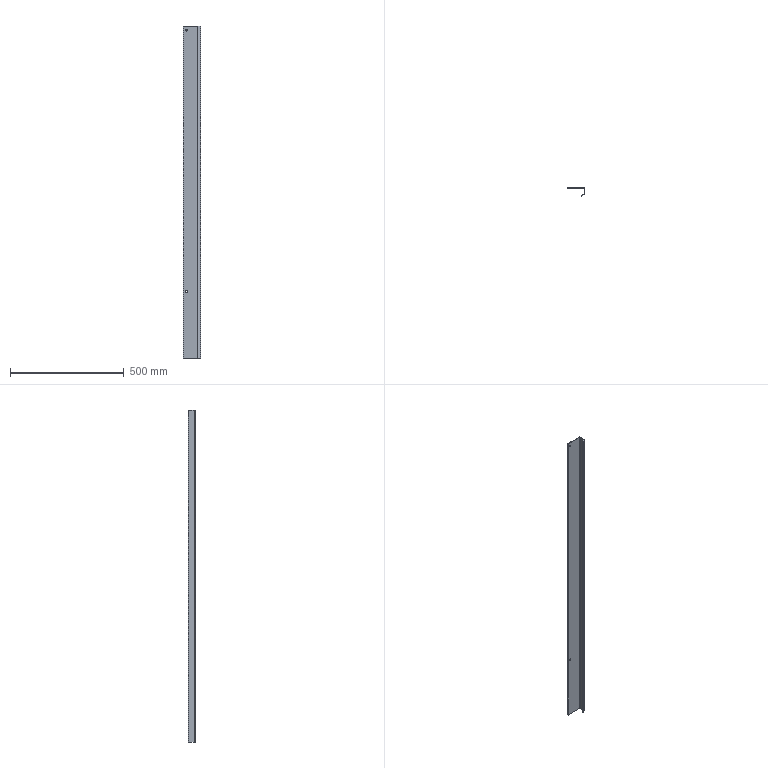Part | STEP file | Guard belt | 1 solid | 20 faces | box 75 x 33.917 x 1461 mm | volume 248061 mm3 | plane 14 | cylinder 6 | commonest cylinder face diameters 3 x2 6 x2 8.2 x2
STEP:
#1=CARTESIAN_POINT('',(0.,0.,0.));
#2=DIRECTION('',(0.,0.,1.));
#3=DIRECTION('',(1.,0.,0.));
#4=AXIS2_PLACEMENT_3D('',#1,#2,#3);
#5=CARTESIAN_POINT('',(-3.,0.,-65.));
#6=VERTEX_POINT('',#5);
#7=CARTESIAN_POINT('',(-3.,1.5,-65.));
#8=VERTEX_POINT('',#7);
#9=CARTESIAN_POINT('',(-3.,0.,-65.));
#10=DIRECTION('',(0.,1.,0.));
#11=VECTOR('',#10,1.);
#12=LINE('',#9,#11);
#13=CARTESIAN_POINT('',(0.,0.,-65.));
#14=DIRECTION('',(0.,0.,1.));
#15=DIRECTION('',(1.,0.,0.));
#16=AXIS2_PLACEMENT_3D('',#13,#14,#15);
#17=PLANE('',#16);
#18=CARTESIAN_POINT('',(-3.,0.));
#19=DIRECTION('',(0.,1.));
#20=VECTOR('',#19,1.);
#21=LINE('',#18,#20);
#22=(GEOMETRIC_REPRESENTATION_CONTEXT(2)PARAMETRIC_REPRESENTATION_CONTEXT()REPRESENTATION_CONTEXT('',''));
#23=DEFINITIONAL_REPRESENTATION('',(#21),#22);
#24=PCURVE('',#17,#23);
#25=CARTESIAN_POINT('',(0.,0.,-65.));
#26=DIRECTION('',(0.,0.,1.));
#27=DIRECTION('',(1.,0.,0.));
#28=AXIS2_PLACEMENT_3D('',#25,#26,#27);
#29=PLANE('',#28);
#30=CARTESIAN_POINT('',(-3.,0.));
#31=DIRECTION('',(0.,1.));
#32=VECTOR('',#31,1.);
#33=LINE('',#30,#32);
#34=(GEOMETRIC_REPRESENTATION_CONTEXT(2)PARAMETRIC_REPRESENTATION_CONTEXT()REPRESENTATION_CONTEXT('',''));
#35=DEFINITIONAL_REPRESENTATION('',(#33),#34);
#36=PCURVE('',#29,#35);
#37=SURFACE_CURVE('',#12,(#24,#36),.PCURVE_S1.);
#38=EDGE_CURVE('',#6,#8,#37,.T.);
#39=ORIENTED_EDGE('',*,*,#38,.F.);
#40=CARTESIAN_POINT('',(-1.5,-1.5,-65.));
#41=VERTEX_POINT('',#40);
#42=CARTESIAN_POINT('',(-3.,-1.5,-65.));
#43=DIRECTION('',(0.,0.,1.));
#44=DIRECTION('',(1.,0.,0.));
#45=AXIS2_PLACEMENT_3D('',#42,#43,#44);
#46=CIRCLE('',#45,1.5);
#47=CARTESIAN_POINT('',(-3.,-1.5));
#48=DIRECTION('',(1.,0.));
#49=AXIS2_PLACEMENT_2D('',#47,#48);
#50=CIRCLE('',#49,1.5);
#51=(GEOMETRIC_REPRESENTATION_CONTEXT(2)PARAMETRIC_REPRESENTATION_CONTEXT()REPRESENTATION_CONTEXT('',''));
#52=DEFINITIONAL_REPRESENTATION('',(#50),#51);
#53=PCURVE('',#17,#52);
#54=CARTESIAN_POINT('',(-3.,-1.5,-913.));
#55=DIRECTION('',(0.,0.,-1.));
#56=DIRECTION('',(0.,1.,0.));
#57=AXIS2_PLACEMENT_3D('',#54,#55,#56);
#58=CYLINDRICAL_SURFACE('',#57,1.5);
#59=CARTESIAN_POINT('',(1.571,-848.));
#60=DIRECTION('',(-1.,0.));
#61=VECTOR('',#60,1.);
#62=LINE('',#59,#61);
#63=(GEOMETRIC_REPRESENTATION_CONTEXT(2)PARAMETRIC_REPRESENTATION_CONTEXT()REPRESENTATION_CONTEXT('',''));
#64=DEFINITIONAL_REPRESENTATION('',(#62),#63);
#65=PCURVE('',#58,#64);
#66=SURFACE_CURVE('',#46,(#53,#65),.PCURVE_S1.);
#67=EDGE_CURVE('',#41,#6,#66,.T.);
#68=ORIENTED_EDGE('',*,*,#67,.F.);
#69=CARTESIAN_POINT('',(0.,-1.5,-65.));
#70=VERTEX_POINT('',#69);
#71=CARTESIAN_POINT('',(-1.17,-1.5,-65.));
#72=DIRECTION('',(-1.,0.,0.));
#73=VECTOR('',#72,1.);
#74=LINE('',#71,#73);
#75=CARTESIAN_POINT('',(-1.17,-1.5));
#76=DIRECTION('',(-1.,0.));
#77=VECTOR('',#76,1.);
#78=LINE('',#75,#77);
#79=(GEOMETRIC_REPRESENTATION_CONTEXT(2)PARAMETRIC_REPRESENTATION_CONTEXT()REPRESENTATION_CONTEXT('',''));
#80=DEFINITIONAL_REPRESENTATION('',(#78),#79);
#81=PCURVE('',#17,#80);
#82=CARTESIAN_POINT('',(0.,0.,-65.));
#83=DIRECTION('',(0.,0.,1.));
#84=DIRECTION('',(1.,0.,0.));
#85=AXIS2_PLACEMENT_3D('',#82,#83,#84);
#86=PLANE('',#85);
#87=CARTESIAN_POINT('',(-1.17,-1.5));
#88=DIRECTION('',(-1.,0.));
#89=VECTOR('',#88,1.);
#90=LINE('',#87,#89);
#91=(GEOMETRIC_REPRESENTATION_CONTEXT(2)PARAMETRIC_REPRESENTATION_CONTEXT()REPRESENTATION_CONTEXT('',''));
#92=DEFINITIONAL_REPRESENTATION('',(#90),#91);
#93=PCURVE('',#86,#92);
#94=SURFACE_CURVE('',#74,(#81,#93),.PCURVE_S1.);
#95=EDGE_CURVE('',#70,#41,#94,.T.);
#96=ORIENTED_EDGE('',*,*,#95,.F.);
#97=CARTESIAN_POINT('',(-3.,-1.5,-65.));
#98=DIRECTION('',(0.,0.,1.));
#99=DIRECTION('',(1.,0.,0.));
#100=AXIS2_PLACEMENT_3D('',#97,#98,#99);
#101=CIRCLE('',#100,3.);
#102=CARTESIAN_POINT('',(-3.,-1.5));
#103=DIRECTION('',(1.,0.));
#104=AXIS2_PLACEMENT_2D('',#102,#103);
#105=CIRCLE('',#104,3.);
#106=(GEOMETRIC_REPRESENTATION_CONTEXT(2)PARAMETRIC_REPRESENTATION_CONTEXT()REPRESENTATION_CONTEXT('',''));
#107=DEFINITIONAL_REPRESENTATION('',(#105),#106);
#108=PCURVE('',#17,#107);
#109=CARTESIAN_POINT('',(-3.,-1.5,-913.));
#110=DIRECTION('',(0.,0.,-1.));
#111=DIRECTION('',(0.,1.,0.));
#112=AXIS2_PLACEMENT_3D('',#109,#110,#111);
#113=CYLINDRICAL_SURFACE('',#112,3.);
#114=CARTESIAN_POINT('',(1.571,-848.));
#115=DIRECTION('',(-1.,0.));
#116=VECTOR('',#115,1.);
#117=LINE('',#114,#116);
#118=(GEOMETRIC_REPRESENTATION_CONTEXT(2)PARAMETRIC_REPRESENTATION_CONTEXT()REPRESENTATION_CONTEXT('',''));
#119=DEFINITIONAL_REPRESENTATION('',(#117),#118);
#120=PCURVE('',#113,#119);
#121=SURFACE_CURVE('',#101,(#108,#120),.PCURVE_S1.);
#122=EDGE_CURVE('',#70,#8,#121,.T.);
#123=ORIENTED_EDGE('',*,*,#122,.T.);
#124=EDGE_LOOP('',(#39,#68,#96,#123));
#125=FACE_BOUND('',#124,.T.);
#126=ADVANCED_FACE('',(#125),#17,.T.);
#127=ORIENTED_EDGE('',*,*,#38,.T.);
#128=CARTESIAN_POINT('',(-75.,1.5,-65.));
#129=VERTEX_POINT('',#128);
#130=CARTESIAN_POINT('',(0.,1.5,-65.));
#131=DIRECTION('',(-1.,0.,0.));
#132=VECTOR('',#131,1.);
#133=LINE('',#130,#132);
#134=CARTESIAN_POINT('',(0.,1.5));
#135=DIRECTION('',(-1.,0.));
#136=VECTOR('',#135,1.);
#137=LINE('',#134,#136);
#138=(GEOMETRIC_REPRESENTATION_CONTEXT(2)PARAMETRIC_REPRESENTATION_CONTEXT()REPRESENTATION_CONTEXT('',''));
#139=DEFINITIONAL_REPRESENTATION('',(#137),#138);
#140=PCURVE('',#29,#139);
#141=CARTESIAN_POINT('',(-37.5,1.5,-913.));
#142=DIRECTION('',(0.,1.,0.));
#143=DIRECTION('',(0.,0.,1.));
#144=AXIS2_PLACEMENT_3D('',#141,#142,#143);
#145=PLANE('',#144);
#146=CARTESIAN_POINT('',(848.,37.5));
#147=DIRECTION('',(0.,-1.));
#148=VECTOR('',#147,1.);
#149=LINE('',#146,#148);
#150=(GEOMETRIC_REPRESENTATION_CONTEXT(2)PARAMETRIC_REPRESENTATION_CONTEXT()REPRESENTATION_CONTEXT('',''));
#151=DEFINITIONAL_REPRESENTATION('',(#149),#150);
#152=PCURVE('',#145,#151);
#153=SURFACE_CURVE('',#133,(#140,#152),.PCURVE_S1.);
#154=EDGE_CURVE('',#8,#129,#153,.T.);
#155=ORIENTED_EDGE('',*,*,#154,.T.);
#156=CARTESIAN_POINT('',(-75.,0.,-65.));
#157=VERTEX_POINT('',#156);
#158=CARTESIAN_POINT('',(-75.,0.,-65.));
#159=DIRECTION('',(0.,1.,0.));
#160=VECTOR('',#159,1.);
#161=LINE('',#158,#160);
#162=CARTESIAN_POINT('',(-75.,0.));
#163=DIRECTION('',(0.,1.));
#164=VECTOR('',#163,1.);
#165=LINE('',#162,#164);
#166=(GEOMETRIC_REPRESENTATION_CONTEXT(2)PARAMETRIC_REPRESENTATION_CONTEXT()REPRESENTATION_CONTEXT('',''));
#167=DEFINITIONAL_REPRESENTATION('',(#165),#166);
#168=PCURVE('',#29,#167);
#169=CARTESIAN_POINT('',(-75.,0.,0.));
#170=DIRECTION('',(-1.,0.,0.));
#171=DIRECTION('',(0.,0.,1.));
#172=AXIS2_PLACEMENT_3D('',#169,#170,#171);
#173=PLANE('',#172);
#174=CARTESIAN_POINT('',(-65.,0.));
#175=DIRECTION('',(0.,1.));
#176=VECTOR('',#175,1.);
#177=LINE('',#174,#176);
#178=(GEOMETRIC_REPRESENTATION_CONTEXT(2)PARAMETRIC_REPRESENTATION_CONTEXT()REPRESENTATION_CONTEXT('',''));
#179=DEFINITIONAL_REPRESENTATION('',(#177),#178);
#180=PCURVE('',#173,#179);
#181=SURFACE_CURVE('',#161,(#168,#180),.PCURVE_S1.);
#182=EDGE_CURVE('',#157,#129,#181,.T.);
#183=ORIENTED_EDGE('',*,*,#182,.F.);
#184=CARTESIAN_POINT('',(0.,0.,-65.));
#185=DIRECTION('',(-1.,0.,0.));
#186=VECTOR('',#185,1.);
#187=LINE('',#184,#186);
#188=CARTESIAN_POINT('',(0.,0.));
#189=DIRECTION('',(-1.,0.));
#190=VECTOR('',#189,1.);
#191=LINE('',#188,#190);
#192=(GEOMETRIC_REPRESENTATION_CONTEXT(2)PARAMETRIC_REPRESENTATION_CONTEXT()REPRESENTATION_CONTEXT('',''));
#193=DEFINITIONAL_REPRESENTATION('',(#191),#192);
#194=PCURVE('',#29,#193);
#195=CARTESIAN_POINT('',(-37.5,0.,-913.));
#196=DIRECTION('',(0.,1.,0.));
#197=DIRECTION('',(0.,0.,1.));
#198=AXIS2_PLACEMENT_3D('',#195,#196,#197);
#199=PLANE('',#198);
#200=CARTESIAN_POINT('',(848.,37.5));
#201=DIRECTION('',(0.,-1.));
#202=VECTOR('',#201,1.);
#203=LINE('',#200,#202);
#204=(GEOMETRIC_REPRESENTATION_CONTEXT(2)PARAMETRIC_REPRESENTATION_CONTEXT()REPRESENTATION_CONTEXT('',''));
#205=DEFINITIONAL_REPRESENTATION('',(#203),#204);
#206=PCURVE('',#199,#205);
#207=SURFACE_CURVE('',#187,(#194,#206),.PCURVE_S1.);
#208=EDGE_CURVE('',#6,#157,#207,.T.);
#209=ORIENTED_EDGE('',*,*,#208,.F.);
#210=EDGE_LOOP('',(#127,#155,#183,#209));
#211=FACE_BOUND('',#210,.T.);
#212=ADVANCED_FACE('',(#211),#29,.T.);
#213=CARTESIAN_POINT('',(-1.5,-24.589,-65.));
#214=VERTEX_POINT('',#213);
#215=CARTESIAN_POINT('',(0.,-24.589,-65.));
#216=VERTEX_POINT('',#215);
#217=CARTESIAN_POINT('',(-1.5,-24.589,-65.));
#218=DIRECTION('',(1.,0.,0.));
#219=VECTOR('',#218,1.);
#220=LINE('',#217,#219);
#221=CARTESIAN_POINT('',(0.,0.,-65.));
#222=DIRECTION('',(0.,0.,1.));
#223=DIRECTION('',(1.,0.,0.));
#224=AXIS2_PLACEMENT_3D('',#221,#222,#223);
#225=PLANE('',#224);
#226=CARTESIAN_POINT('',(-1.5,-24.589));
#227=DIRECTION('',(1.,0.));
#228=VECTOR('',#227,1.);
#229=LINE('',#226,#228);
#230=(GEOMETRIC_REPRESENTATION_CONTEXT(2)PARAMETRIC_REPRESENTATION_CONTEXT()REPRESENTATION_CONTEXT('',''));
#231=DEFINITIONAL_REPRESENTATION('',(#229),#230);
#232=PCURVE('',#225,#231);
#233=CARTESIAN_POINT('',(-1.5,-24.589));
#234=DIRECTION('',(1.,0.));
#235=VECTOR('',#234,1.);
#236=LINE('',#233,#235);
#237=(GEOMETRIC_REPRESENTATION_CONTEXT(2)PARAMETRIC_REPRESENTATION_CONTEXT()REPRESENTATION_CONTEXT('',''));
#238=DEFINITIONAL_REPRESENTATION('',(#236),#237);
#239=PCURVE('',#86,#238);
#240=SURFACE_CURVE('',#220,(#232,#239),.PCURVE_S1.);
#241=EDGE_CURVE('',#214,#216,#240,.T.);
#242=ORIENTED_EDGE('',*,*,#241,.F.);
#243=CARTESIAN_POINT('',(-2.366,-25.948,-65.));
#244=VERTEX_POINT('',#243);
#245=CARTESIAN_POINT('',(-3.,-24.589,-65.));
#246=DIRECTION('',(0.,0.,1.));
#247=DIRECTION('',(0.4226,-0.9063,0.));
#248=AXIS2_PLACEMENT_3D('',#245,#246,#247);
#249=CIRCLE('',#248,1.5);
#250=CARTESIAN_POINT('',(-3.,-24.589));
#251=DIRECTION('',(0.4226,-0.9063));
#252=AXIS2_PLACEMENT_2D('',#250,#251);
#253=CIRCLE('',#252,1.5);
#254=(GEOMETRIC_REPRESENTATION_CONTEXT(2)PARAMETRIC_REPRESENTATION_CONTEXT()REPRESENTATION_CONTEXT('',''));
#255=DEFINITIONAL_REPRESENTATION('',(#253),#254);
#256=PCURVE('',#225,#255);
#257=CARTESIAN_POINT('',(-3.,-24.589,-913.));
#258=DIRECTION('',(0.,0.,-1.));
#259=DIRECTION('',(1.,0.,0.));
#260=AXIS2_PLACEMENT_3D('',#257,#258,#259);
#261=CYLINDRICAL_SURFACE('',#260,1.5);
#262=CARTESIAN_POINT('',(1.134,-848.));
#263=DIRECTION('',(-1.,0.));
#264=VECTOR('',#263,1.);
#265=LINE('',#262,#264);
#266=(GEOMETRIC_REPRESENTATION_CONTEXT(2)PARAMETRIC_REPRESENTATION_CONTEXT()REPRESENTATION_CONTEXT('',''));
#267=DEFINITIONAL_REPRESENTATION('',(#265),#266);
#268=PCURVE('',#261,#267);
#269=SURFACE_CURVE('',#249,(#256,#268),.PCURVE_S1.);
#270=EDGE_CURVE('',#244,#214,#269,.T.);
#271=ORIENTED_EDGE('',*,*,#270,.F.);
#272=CARTESIAN_POINT('',(-1.732,-27.308,-65.));
#273=VERTEX_POINT('',#272);
#274=CARTESIAN_POINT('',(-2.227,-26.247,-65.));
#275=DIRECTION('',(-0.4226,0.9063,0.));
#276=VECTOR('',#275,1.);
#277=LINE('',#274,#276);
#278=CARTESIAN_POINT('',(-2.227,-26.247));
#279=DIRECTION('',(-0.4226,0.9063));
#280=VECTOR('',#279,1.);
#281=LINE('',#278,#280);
#282=(GEOMETRIC_REPRESENTATION_CONTEXT(2)PARAMETRIC_REPRESENTATION_CONTEXT()REPRESENTATION_CONTEXT('',''));
#283=DEFINITIONAL_REPRESENTATION('',(#281),#282);
#284=PCURVE('',#225,#283);
#285=CARTESIAN_POINT('',(0.,0.,-65.));
#286=DIRECTION('',(0.,0.,1.));
#287=DIRECTION('',(1.,0.,0.));
#288=AXIS2_PLACEMENT_3D('',#285,#286,#287);
#289=PLANE('',#288);
#290=CARTESIAN_POINT('',(-2.227,-26.247));
#291=DIRECTION('',(-0.4226,0.9063));
#292=VECTOR('',#291,1.);
#293=LINE('',#290,#292);
#294=(GEOMETRIC_REPRESENTATION_CONTEXT(2)PARAMETRIC_REPRESENTATION_CONTEXT()REPRESENTATION_CONTEXT('',''));
#295=DEFINITIONAL_REPRESENTATION('',(#293),#294);
#296=PCURVE('',#289,#295);
#297=SURFACE_CURVE('',#277,(#284,#296),.PCURVE_S1.);
#298=EDGE_CURVE('',#273,#244,#297,.T.);
#299=ORIENTED_EDGE('',*,*,#298,.F.);
#300=CARTESIAN_POINT('',(-3.,-24.589,-65.));
#301=DIRECTION('',(0.,0.,1.));
#302=DIRECTION('',(0.4226,-0.9063,0.));
#303=AXIS2_PLACEMENT_3D('',#300,#301,#302);
#304=CIRCLE('',#303,3.);
#305=CARTESIAN_POINT('',(-3.,-24.589));
#306=DIRECTION('',(0.4226,-0.9063));
#307=AXIS2_PLACEMENT_2D('',#305,#306);
#308=CIRCLE('',#307,3.);
#309=(GEOMETRIC_REPRESENTATION_CONTEXT(2)PARAMETRIC_REPRESENTATION_CONTEXT()REPRESENTATION_CONTEXT('',''));
#310=DEFINITIONAL_REPRESENTATION('',(#308),#309);
#311=PCURVE('',#225,#310);
#312=CARTESIAN_POINT('',(-3.,-24.589,-913.));
#313=DIRECTION('',(0.,0.,-1.));
#314=DIRECTION('',(1.,0.,0.));
#315=AXIS2_PLACEMENT_3D('',#312,#313,#314);
#316=CYLINDRICAL_SURFACE('',#315,3.);
#317=CARTESIAN_POINT('',(1.134,-848.));
#318=DIRECTION('',(-1.,0.));
#319=VECTOR('',#318,1.);
#320=LINE('',#317,#319);
#321=(GEOMETRIC_REPRESENTATION_CONTEXT(2)PARAMETRIC_REPRESENTATION_CONTEXT()REPRESENTATION_CONTEXT('',''));
#322=DEFINITIONAL_REPRESENTATION('',(#320),#321);
#323=PCURVE('',#316,#322);
#324=SURFACE_CURVE('',#304,(#311,#323),.PCURVE_S1.);
#325=EDGE_CURVE('',#273,#216,#324,.T.);
#326=ORIENTED_EDGE('',*,*,#325,.T.);
#327=EDGE_LOOP('',(#242,#271,#299,#326));
#328=FACE_BOUND('',#327,.T.);
#329=ADVANCED_FACE('',(#328),#225,.T.);
#330=ORIENTED_EDGE('',*,*,#95,.T.);
#331=CARTESIAN_POINT('',(-1.5,5.286,-65.));
#332=DIRECTION('',(0.,1.,0.));
#333=VECTOR('',#332,1.);
#334=LINE('',#331,#333);
#335=CARTESIAN_POINT('',(-1.5,5.286));
#336=DIRECTION('',(0.,1.));
#337=VECTOR('',#336,1.);
#338=LINE('',#335,#337);
#339=(GEOMETRIC_REPRESENTATION_CONTEXT(2)PARAMETRIC_REPRESENTATION_CONTEXT()REPRESENTATION_CONTEXT('',''));
#340=DEFINITIONAL_REPRESENTATION('',(#338),#339);
#341=PCURVE('',#86,#340);
#342=CARTESIAN_POINT('',(-1.5,-12.304,-913.));
#343=DIRECTION('',(1.,0.,0.));
#344=DIRECTION('',(0.,0.,1.));
#345=AXIS2_PLACEMENT_3D('',#342,#343,#344);
#346=PLANE('',#345);
#347=CARTESIAN_POINT('',(848.,-17.589));
#348=DIRECTION('',(0.,-1.));
#349=VECTOR('',#348,1.);
#350=LINE('',#347,#349);
#351=(GEOMETRIC_REPRESENTATION_CONTEXT(2)PARAMETRIC_REPRESENTATION_CONTEXT()REPRESENTATION_CONTEXT('',''));
#352=DEFINITIONAL_REPRESENTATION('',(#350),#351);
#353=PCURVE('',#346,#352);
#354=SURFACE_CURVE('',#334,(#341,#353),.PCURVE_S1.);
#355=EDGE_CURVE('',#214,#41,#354,.T.);
#356=ORIENTED_EDGE('',*,*,#355,.F.);
#357=ORIENTED_EDGE('',*,*,#241,.T.);
#358=CARTESIAN_POINT('',(0.,5.286,-65.));
#359=DIRECTION('',(0.,1.,0.));
#360=VECTOR('',#359,1.);
#361=LINE('',#358,#360);
#362=CARTESIAN_POINT('',(0.,5.286));
#363=DIRECTION('',(0.,1.));
#364=VECTOR('',#363,1.);
#365=LINE('',#362,#364);
#366=(GEOMETRIC_REPRESENTATION_CONTEXT(2)PARAMETRIC_REPRESENTATION_CONTEXT()REPRESENTATION_CONTEXT('',''));
#367=DEFINITIONAL_REPRESENTATION('',(#365),#366);
#368=PCURVE('',#86,#367);
#369=CARTESIAN_POINT('',(0.,-12.304,-913.));
#370=DIRECTION('',(1.,0.,0.));
#371=DIRECTION('',(0.,0.,1.));
#372=AXIS2_PLACEMENT_3D('',#369,#370,#371);
#373=PLANE('',#372);
#374=CARTESIAN_POINT('',(848.,-17.589));
#375=DIRECTION('',(0.,-1.));
#376=VECTOR('',#375,1.);
#377=LINE('',#374,#376);
#378=(GEOMETRIC_REPRESENTATION_CONTEXT(2)PARAMETRIC_REPRESENTATION_CONTEXT()REPRESENTATION_CONTEXT('',''));
#379=DEFINITIONAL_REPRESENTATION('',(#377),#378);
#380=PCURVE('',#373,#379);
#381=SURFACE_CURVE('',#361,(#368,#380),.PCURVE_S1.);
#382=EDGE_CURVE('',#216,#70,#381,.T.);
#383=ORIENTED_EDGE('',*,*,#382,.T.);
#384=EDGE_LOOP('',(#330,#356,#357,#383));
#385=FACE_BOUND('',#384,.T.);
#386=ADVANCED_FACE('',(#385),#86,.T.);
#387=CARTESIAN_POINT('',(-57.4,0.,-1233.5));
#388=VERTEX_POINT('',#387);
#389=CARTESIAN_POINT('',(-61.5,0.,-1233.5));
#390=DIRECTION('',(0.,1.,0.));
#391=DIRECTION('',(-1.,0.,0.));
#392=AXIS2_PLACEMENT_3D('',#389,#390,#391);
#393=CIRCLE('',#392,4.1);
#394=CARTESIAN_POINT('',(-61.5,1.5,-1233.5));
#395=DIRECTION('',(0.,-1.,0.));
#396=DIRECTION('',(-1.,0.,0.));
#397=AXIS2_PLACEMENT_3D('',#394,#395,#396);
#398=CYLINDRICAL_SURFACE('',#397,4.1);
#399=CARTESIAN_POINT('',(12.566,1.5));
#400=DIRECTION('',(-1.,0.));
#401=VECTOR('',#400,1.);
#402=LINE('',#399,#401);
#403=(GEOMETRIC_REPRESENTATION_CONTEXT(2)PARAMETRIC_REPRESENTATION_CONTEXT()REPRESENTATION_CONTEXT('',''));
#404=DEFINITIONAL_REPRESENTATION('',(#402),#403);
#405=PCURVE('',#398,#404);
#406=CARTESIAN_POINT('',(-320.5,-24.));
#407=DIRECTION('',(0.,-1.));
#408=AXIS2_PLACEMENT_2D('',#406,#407);
#409=CIRCLE('',#408,4.1);
#410=(GEOMETRIC_REPRESENTATION_CONTEXT(2)PARAMETRIC_REPRESENTATION_CONTEXT()REPRESENTATION_CONTEXT('',''));
#411=DEFINITIONAL_REPRESENTATION('',(#409),#410);
#412=PCURVE('',#199,#411);
#413=SURFACE_CURVE('',#393,(#405,#412),.PCURVE_S1.);
#414=EDGE_CURVE('',#388,#388,#413,.T.);
#415=ORIENTED_EDGE('',*,*,#414,.T.);
#416=CARTESIAN_POINT('',(-57.4,1.5,-1233.5));
#417=VERTEX_POINT('',#416);
#418=CARTESIAN_POINT('',(-57.4,1.5,-1233.5));
#419=CARTESIAN_POINT('',(-57.4,0.,-1233.5));
#420=B_SPLINE_CURVE_WITH_KNOTS('',1,(#418,#419),.UNSPECIFIED.,.F.,.F.,(2,2),(0.,1.5),.PIECEWISE_BEZIER_KNOTS.);
#421=CARTESIAN_POINT('',(3.142,0.));
#422=DIRECTION('',(0.,1.));
#423=VECTOR('',#422,1.);
#424=LINE('',#421,#423);
#425=(GEOMETRIC_REPRESENTATION_CONTEXT(2)PARAMETRIC_REPRESENTATION_CONTEXT()REPRESENTATION_CONTEXT('',''));
#426=DEFINITIONAL_REPRESENTATION('',(#424),#425);
#427=PCURVE('',#398,#426);
#428=CARTESIAN_POINT('',(9.425,0.));
#429=DIRECTION('',(0.,1.));
#430=VECTOR('',#429,1.);
#431=LINE('',#428,#430);
#432=(GEOMETRIC_REPRESENTATION_CONTEXT(2)PARAMETRIC_REPRESENTATION_CONTEXT()REPRESENTATION_CONTEXT('',''));
#433=DEFINITIONAL_REPRESENTATION('',(#431),#432);
#434=PCURVE('',#398,#433);
#435=SEAM_CURVE('',#420,(#427,#434),.PCURVE_S1.);
#436=EDGE_CURVE('',#417,#388,#435,.T.);
#437=ORIENTED_EDGE('',*,*,#436,.F.);
#438=CARTESIAN_POINT('',(-61.5,1.5,-1233.5));
#439=DIRECTION('',(0.,-1.,0.));
#440=DIRECTION('',(-1.,0.,0.));
#441=AXIS2_PLACEMENT_3D('',#438,#439,#440);
#442=CIRCLE('',#441,4.1);
#443=CARTESIAN_POINT('',(0.,0.));
#444=DIRECTION('',(1.,0.));
#445=VECTOR('',#444,1.);
#446=LINE('',#443,#445);
#447=(GEOMETRIC_REPRESENTATION_CONTEXT(2)PARAMETRIC_REPRESENTATION_CONTEXT()REPRESENTATION_CONTEXT('',''));
#448=DEFINITIONAL_REPRESENTATION('',(#446),#447);
#449=PCURVE('',#398,#448);
#450=CARTESIAN_POINT('',(-320.5,-28.1));
#451=CARTESIAN_POINT('',(-327.601,-28.1));
#452=CARTESIAN_POINT('',(-324.051,-21.95));
#453=CARTESIAN_POINT('',(-320.5,-15.8));
#454=CARTESIAN_POINT('',(-316.949,-21.95));
#455=CARTESIAN_POINT('',(-313.399,-28.1));
#456=CARTESIAN_POINT('',(-320.5,-28.1));
#457=(BOUNDED_CURVE()B_SPLINE_CURVE(2,(#450,#451,#452,#453,#454,#455,#456),.UNSPECIFIED.,.T.,.F.)B_SPLINE_CURVE_WITH_KNOTS((1,2,2,2,2,1),(-2.094,0.,2.094,4.189,6.283,8.378),.UNSPECIFIED.)CURVE()GEOMETRIC_REPRESENTATION_ITEM()RATIONAL_B_SPLINE_CURVE((1.,0.5,1.,0.5,1.,0.5,1.))REPRESENTATION_ITEM(''));
#458=(GEOMETRIC_REPRESENTATION_CONTEXT(2)PARAMETRIC_REPRESENTATION_CONTEXT()REPRESENTATION_CONTEXT('',''));
#459=DEFINITIONAL_REPRESENTATION('',(#457),#458);
#460=PCURVE('',#145,#459);
#461=SURFACE_CURVE('',#442,(#449,#460),.PCURVE_S1.);
#462=EDGE_CURVE('',#417,#417,#461,.T.);
#463=ORIENTED_EDGE('',*,*,#462,.T.);
#464=ORIENTED_EDGE('',*,*,#436,.T.);
#465=EDGE_LOOP('',(#415,#437,#463,#464));
#466=FACE_BOUND('',#465,.F.);
#467=ADVANCED_FACE('',(#466),#398,.F.);
#468=CARTESIAN_POINT('',(-57.4,0.,-83.5));
#469=VERTEX_POINT('',#468);
#470=CARTESIAN_POINT('',(-61.5,0.,-83.5));
#471=DIRECTION('',(0.,1.,0.));
#472=DIRECTION('',(-1.,0.,0.));
#473=AXIS2_PLACEMENT_3D('',#470,#471,#472);
#474=CIRCLE('',#473,4.1);
#475=CARTESIAN_POINT('',(-61.5,1.5,-83.5));
#476=DIRECTION('',(0.,-1.,0.));
#477=DIRECTION('',(-1.,0.,0.));
#478=AXIS2_PLACEMENT_3D('',#475,#476,#477);
#479=CYLINDRICAL_SURFACE('',#478,4.1);
#480=CARTESIAN_POINT('',(12.566,1.5));
#481=DIRECTION('',(-1.,0.));
#482=VECTOR('',#481,1.);
#483=LINE('',#480,#482);
#484=(GEOMETRIC_REPRESENTATION_CONTEXT(2)PARAMETRIC_REPRESENTATION_CONTEXT()REPRESENTATION_CONTEXT('',''));
#485=DEFINITIONAL_REPRESENTATION('',(#483),#484);
#486=PCURVE('',#479,#485);
#487=CARTESIAN_POINT('',(829.5,-24.));
#488=DIRECTION('',(0.,-1.));
#489=AXIS2_PLACEMENT_2D('',#487,#488);
#490=CIRCLE('',#489,4.1);
#491=(GEOMETRIC_REPRESENTATION_CONTEXT(2)PARAMETRIC_REPRESENTATION_CONTEXT()REPRESENTATION_CONTEXT('',''));
#492=DEFINITIONAL_REPRESENTATION('',(#490),#491);
#493=PCURVE('',#199,#492);
#494=SURFACE_CURVE('',#474,(#486,#493),.PCURVE_S1.);
#495=EDGE_CURVE('',#469,#469,#494,.T.);
#496=ORIENTED_EDGE('',*,*,#495,.T.);
#497=CARTESIAN_POINT('',(-57.4,1.5,-83.5));
#498=VERTEX_POINT('',#497);
#499=CARTESIAN_POINT('',(-57.4,1.5,-83.5));
#500=CARTESIAN_POINT('',(-57.4,0.,-83.5));
#501=B_SPLINE_CURVE_WITH_KNOTS('',1,(#499,#500),.UNSPECIFIED.,.F.,.F.,(2,2),(0.,1.5),.PIECEWISE_BEZIER_KNOTS.);
#502=CARTESIAN_POINT('',(3.142,0.));
#503=DIRECTION('',(0.,1.));
#504=VECTOR('',#503,1.);
#505=LINE('',#502,#504);
#506=(GEOMETRIC_REPRESENTATION_CONTEXT(2)PARAMETRIC_REPRESENTATION_CONTEXT()REPRESENTATION_CONTEXT('',''));
#507=DEFINITIONAL_REPRESENTATION('',(#505),#506);
#508=PCURVE('',#479,#507);
#509=CARTESIAN_POINT('',(9.425,0.));
#510=DIRECTION('',(0.,1.));
#511=VECTOR('',#510,1.);
#512=LINE('',#509,#511);
#513=(GEOMETRIC_REPRESENTATION_CONTEXT(2)PARAMETRIC_REPRESENTATION_CONTEXT()REPRESENTATION_CONTEXT('',''));
#514=DEFINITIONAL_REPRESENTATION('',(#512),#513);
#515=PCURVE('',#479,#514);
#516=SEAM_CURVE('',#501,(#508,#515),.PCURVE_S1.);
#517=EDGE_CURVE('',#498,#469,#516,.T.);
#518=ORIENTED_EDGE('',*,*,#517,.F.);
#519=CARTESIAN_POINT('',(-61.5,1.5,-83.5));
#520=DIRECTION('',(0.,-1.,0.));
#521=DIRECTION('',(-1.,0.,0.));
#522=AXIS2_PLACEMENT_3D('',#519,#520,#521);
#523=CIRCLE('',#522,4.1);
#524=CARTESIAN_POINT('',(0.,0.));
#525=DIRECTION('',(1.,0.));
#526=VECTOR('',#525,1.);
#527=LINE('',#524,#526);
#528=(GEOMETRIC_REPRESENTATION_CONTEXT(2)PARAMETRIC_REPRESENTATION_CONTEXT()REPRESENTATION_CONTEXT('',''));
#529=DEFINITIONAL_REPRESENTATION('',(#527),#528);
#530=PCURVE('',#479,#529);
#531=CARTESIAN_POINT('',(829.5,-28.1));
#532=CARTESIAN_POINT('',(822.399,-28.1));
#533=CARTESIAN_POINT('',(825.949,-21.95));
#534=CARTESIAN_POINT('',(829.5,-15.8));
#535=CARTESIAN_POINT('',(833.051,-21.95));
#536=CARTESIAN_POINT('',(836.601,-28.1));
#537=CARTESIAN_POINT('',(829.5,-28.1));
#538=(BOUNDED_CURVE()B_SPLINE_CURVE(2,(#531,#532,#533,#534,#535,#536,#537),.UNSPECIFIED.,.T.,.F.)B_SPLINE_CURVE_WITH_KNOTS((1,2,2,2,2,1),(-2.094,0.,2.094,4.189,6.283,8.378),.UNSPECIFIED.)CURVE()GEOMETRIC_REPRESENTATION_ITEM()RATIONAL_B_SPLINE_CURVE((1.,0.5,1.,0.5,1.,0.5,1.))REPRESENTATION_ITEM(''));
#539=(GEOMETRIC_REPRESENTATION_CONTEXT(2)PARAMETRIC_REPRESENTATION_CONTEXT()REPRESENTATION_CONTEXT('',''));
#540=DEFINITIONAL_REPRESENTATION('',(#538),#539);
#541=PCURVE('',#145,#540);
#542=SURFACE_CURVE('',#523,(#530,#541),.PCURVE_S1.);
#543=EDGE_CURVE('',#498,#498,#542,.T.);
#544=ORIENTED_EDGE('',*,*,#543,.T.);
#545=ORIENTED_EDGE('',*,*,#517,.T.);
#546=EDGE_LOOP('',(#496,#518,#544,#545));
#547=FACE_BOUND('',#546,.F.);
#548=ADVANCED_FACE('',(#547),#479,.F.);
#549=CARTESIAN_POINT('',(-75.,1.5,-1526.));
#550=VERTEX_POINT('',#549);
#551=CARTESIAN_POINT('',(-75.,0.,-1526.));
#552=VERTEX_POINT('',#551);
#553=CARTESIAN_POINT('',(-75.,0.75,-1526.));
#554=DIRECTION('',(0.,-1.,0.));
#555=VECTOR('',#554,1.);
#556=LINE('',#553,#555);
#557=CARTESIAN_POINT('',(15.619,1.5,-1526.));
#558=DIRECTION('',(0.,0.,1.));
#559=DIRECTION('',(-1.,0.,0.));
#560=AXIS2_PLACEMENT_3D('',#557,#558,#559);
#561=PLANE('',#560);
#562=CARTESIAN_POINT('',(90.619,0.75));
#563=DIRECTION('',(0.,1.));
#564=VECTOR('',#563,1.);
#565=LINE('',#562,#564);
#566=(GEOMETRIC_REPRESENTATION_CONTEXT(2)PARAMETRIC_REPRESENTATION_CONTEXT()REPRESENTATION_CONTEXT('',''));
#567=DEFINITIONAL_REPRESENTATION('',(#565),#566);
#568=PCURVE('',#561,#567);
#569=CARTESIAN_POINT('',(-1526.,0.75));
#570=DIRECTION('',(0.,-1.));
#571=VECTOR('',#570,1.);
#572=LINE('',#569,#571);
#573=(GEOMETRIC_REPRESENTATION_CONTEXT(2)PARAMETRIC_REPRESENTATION_CONTEXT()REPRESENTATION_CONTEXT('',''));
#574=DEFINITIONAL_REPRESENTATION('',(#572),#573);
#575=PCURVE('',#173,#574);
#576=SURFACE_CURVE('',#556,(#568,#575),.PCURVE_S1.);
#577=EDGE_CURVE('',#550,#552,#576,.T.);
#578=ORIENTED_EDGE('',*,*,#577,.F.);
#579=CARTESIAN_POINT('',(-3.,1.5,-1526.));
#580=VERTEX_POINT('',#579);
#581=CARTESIAN_POINT('',(-10.941,1.5,-1526.));
#582=DIRECTION('',(-1.,0.,0.));
#583=VECTOR('',#582,1.);
#584=LINE('',#581,#583);
#585=CARTESIAN_POINT('',(26.559,0.));
#586=DIRECTION('',(1.,0.));
#587=VECTOR('',#586,1.);
#588=LINE('',#585,#587);
#589=(GEOMETRIC_REPRESENTATION_CONTEXT(2)PARAMETRIC_REPRESENTATION_CONTEXT()REPRESENTATION_CONTEXT('',''));
#590=DEFINITIONAL_REPRESENTATION('',(#588),#589);
#591=PCURVE('',#561,#590);
#592=CARTESIAN_POINT('',(-613.,26.559));
#593=DIRECTION('',(0.,-1.));
#594=VECTOR('',#593,1.);
#595=LINE('',#592,#594);
#596=(GEOMETRIC_REPRESENTATION_CONTEXT(2)PARAMETRIC_REPRESENTATION_CONTEXT()REPRESENTATION_CONTEXT('',''));
#597=DEFINITIONAL_REPRESENTATION('',(#595),#596);
#598=PCURVE('',#145,#597);
#599=SURFACE_CURVE('',#584,(#591,#598),.PCURVE_S1.);
#600=EDGE_CURVE('',#580,#550,#599,.T.);
#601=ORIENTED_EDGE('',*,*,#600,.F.);
#602=CARTESIAN_POINT('',(0.,-1.5,-1526.));
#603=VERTEX_POINT('',#602);
#604=CARTESIAN_POINT('',(-3.,-1.5,-1526.));
#605=DIRECTION('',(0.,0.,1.));
#606=DIRECTION('',(0.,1.,0.));
#607=AXIS2_PLACEMENT_3D('',#604,#605,#606);
#608=CIRCLE('',#607,3.);
#609=CARTESIAN_POINT('',(18.619,3.));
#610=DIRECTION('',(0.,-1.));
#611=AXIS2_PLACEMENT_2D('',#609,#610);
#612=CIRCLE('',#611,3.);
#613=(GEOMETRIC_REPRESENTATION_CONTEXT(2)PARAMETRIC_REPRESENTATION_CONTEXT()REPRESENTATION_CONTEXT('',''));
#614=DEFINITIONAL_REPRESENTATION('',(#612),#613);
#615=PCURVE('',#561,#614);
#616=CARTESIAN_POINT('',(6.283,613.));
#617=DIRECTION('',(-1.,0.));
#618=VECTOR('',#617,1.);
#619=LINE('',#616,#618);
#620=(GEOMETRIC_REPRESENTATION_CONTEXT(2)PARAMETRIC_REPRESENTATION_CONTEXT()REPRESENTATION_CONTEXT('',''));
#621=DEFINITIONAL_REPRESENTATION('',(#619),#620);
#622=PCURVE('',#113,#621);
#623=SURFACE_CURVE('',#608,(#615,#622),.PCURVE_S1.);
#624=EDGE_CURVE('',#603,#580,#623,.T.);
#625=ORIENTED_EDGE('',*,*,#624,.F.);
#626=CARTESIAN_POINT('',(0.,-24.589,-1526.));
#627=VERTEX_POINT('',#626);
#628=CARTESIAN_POINT('',(0.,-5.402,-1526.));
#629=DIRECTION('',(0.,1.,0.));
#630=VECTOR('',#629,1.);
#631=LINE('',#628,#630);
#632=CARTESIAN_POINT('',(15.619,6.902));
#633=DIRECTION('',(0.,-1.));
#634=VECTOR('',#633,1.);
#635=LINE('',#632,#634);
#636=(GEOMETRIC_REPRESENTATION_CONTEXT(2)PARAMETRIC_REPRESENTATION_CONTEXT()REPRESENTATION_CONTEXT('',''));
#637=DEFINITIONAL_REPRESENTATION('',(#635),#636);
#638=PCURVE('',#561,#637);
#639=CARTESIAN_POINT('',(-613.,-6.902));
#640=DIRECTION('',(0.,-1.));
#641=VECTOR('',#640,1.);
#642=LINE('',#639,#641);
#643=(GEOMETRIC_REPRESENTATION_CONTEXT(2)PARAMETRIC_REPRESENTATION_CONTEXT()REPRESENTATION_CONTEXT('',''));
#644=DEFINITIONAL_REPRESENTATION('',(#642),#643);
#645=PCURVE('',#373,#644);
#646=SURFACE_CURVE('',#631,(#638,#645),.PCURVE_S1.);
#647=EDGE_CURVE('',#627,#603,#646,.T.);
#648=ORIENTED_EDGE('',*,*,#647,.F.);
#649=CARTESIAN_POINT('',(-1.732,-27.308,-1526.));
#650=VERTEX_POINT('',#649);
#651=CARTESIAN_POINT('',(-3.,-24.589,-1526.));
#652=DIRECTION('',(0.,0.,1.));
#653=DIRECTION('',(1.,0.,0.));
#654=AXIS2_PLACEMENT_3D('',#651,#652,#653);
#655=CIRCLE('',#654,3.);
#656=CARTESIAN_POINT('',(18.619,26.089));
#657=DIRECTION('',(-1.,0.));
#658=AXIS2_PLACEMENT_2D('',#656,#657);
#659=CIRCLE('',#658,3.);
#660=(GEOMETRIC_REPRESENTATION_CONTEXT(2)PARAMETRIC_REPRESENTATION_CONTEXT()REPRESENTATION_CONTEXT('',''));
#661=DEFINITIONAL_REPRESENTATION('',(#659),#660);
#662=PCURVE('',#561,#661);
#663=CARTESIAN_POINT('',(6.283,613.));
#664=DIRECTION('',(-1.,0.));
#665=VECTOR('',#664,1.);
#666=LINE('',#663,#665);
#667=(GEOMETRIC_REPRESENTATION_CONTEXT(2)PARAMETRIC_REPRESENTATION_CONTEXT()REPRESENTATION_CONTEXT('',''));
#668=DEFINITIONAL_REPRESENTATION('',(#666),#667);
#669=PCURVE('',#316,#668);
#670=SURFACE_CURVE('',#655,(#662,#669),.PCURVE_S1.);
#671=EDGE_CURVE('',#650,#627,#670,.T.);
#672=ORIENTED_EDGE('',*,*,#671,.F.);
#673=CARTESIAN_POINT('',(-12.688,-32.417,-1526.));
#674=VERTEX_POINT('',#673);
#675=CARTESIAN_POINT('',(8.727,-22.431,-1526.));
#676=DIRECTION('',(0.9063,0.4226,0.));
#677=VECTOR('',#676,1.);
#678=LINE('',#675,#677);
#679=CARTESIAN_POINT('',(6.892,23.931));
#680=DIRECTION('',(-0.9063,-0.4226));
#681=VECTOR('',#680,1.);
#682=LINE('',#679,#681);
#683=(GEOMETRIC_REPRESENTATION_CONTEXT(2)PARAMETRIC_REPRESENTATION_CONTEXT()REPRESENTATION_CONTEXT('',''));
#684=DEFINITIONAL_REPRESENTATION('',(#682),#683);
#685=PCURVE('',#561,#684);
#686=CARTESIAN_POINT('',(-6.1,-29.344,-913.));
#687=DIRECTION('',(0.4226,-0.9063,0.));
#688=DIRECTION('',(0.,0.,-1.));
#689=AXIS2_PLACEMENT_3D('',#686,#687,#688);
#690=PLANE('',#689);
#691=CARTESIAN_POINT('',(613.,16.36));
#692=DIRECTION('',(0.,1.));
#693=VECTOR('',#692,1.);
#694=LINE('',#691,#693);
#695=(GEOMETRIC_REPRESENTATION_CONTEXT(2)PARAMETRIC_REPRESENTATION_CONTEXT()REPRESENTATION_CONTEXT('',''));
#696=DEFINITIONAL_REPRESENTATION('',(#694),#695);
#697=PCURVE('',#690,#696);
#698=SURFACE_CURVE('',#678,(#685,#697),.PCURVE_S1.);
#699=EDGE_CURVE('',#674,#650,#698,.T.);
#700=ORIENTED_EDGE('',*,*,#699,.F.);
#701=CARTESIAN_POINT('',(-13.322,-31.057,-1526.));
#702=VERTEX_POINT('',#701);
#703=CARTESIAN_POINT('',(-16.973,-23.229,-1526.));
#704=DIRECTION('',(0.4226,-0.9063,0.));
#705=VECTOR('',#704,1.);
#706=LINE('',#703,#705);
#707=CARTESIAN_POINT('',(32.591,24.729));
#708=DIRECTION('',(-0.4226,0.9063));
#709=VECTOR('',#708,1.);
#710=LINE('',#707,#709);
#711=(GEOMETRIC_REPRESENTATION_CONTEXT(2)PARAMETRIC_REPRESENTATION_CONTEXT()REPRESENTATION_CONTEXT('',''));
#712=DEFINITIONAL_REPRESENTATION('',(#710),#711);
#713=PCURVE('',#561,#712);
#714=CARTESIAN_POINT('',(-13.322,-31.057,-1826.));
#715=DIRECTION('',(-0.9063,-0.4226,0.));
#716=DIRECTION('',(0.,0.,-1.));
#717=AXIS2_PLACEMENT_3D('',#714,#715,#716);
#718=PLANE('',#717);
#719=CARTESIAN_POINT('',(-300.,-8.638));
#720=DIRECTION('',(0.,1.));
#721=VECTOR('',#720,1.);
#722=LINE('',#719,#721);
#723=(GEOMETRIC_REPRESENTATION_CONTEXT(2)PARAMETRIC_REPRESENTATION_CONTEXT()REPRESENTATION_CONTEXT('',''));
#724=DEFINITIONAL_REPRESENTATION('',(#722),#723);
#725=PCURVE('',#718,#724);
#726=SURFACE_CURVE('',#706,(#713,#725),.PCURVE_S1.);
#727=EDGE_CURVE('',#702,#674,#726,.T.);
#728=ORIENTED_EDGE('',*,*,#727,.F.);
#729=CARTESIAN_POINT('',(-2.366,-25.948,-1526.));
#730=VERTEX_POINT('',#729);
#731=CARTESIAN_POINT('',(8.093,-21.071,-1526.));
#732=DIRECTION('',(-0.9063,-0.4226,0.));
#733=VECTOR('',#732,1.);
#734=LINE('',#731,#733);
#735=CARTESIAN_POINT('',(7.526,22.571));
#736=DIRECTION('',(0.9063,0.4226));
#737=VECTOR('',#736,1.);
#738=LINE('',#735,#737);
#739=(GEOMETRIC_REPRESENTATION_CONTEXT(2)PARAMETRIC_REPRESENTATION_CONTEXT()REPRESENTATION_CONTEXT('',''));
#740=DEFINITIONAL_REPRESENTATION('',(#738),#739);
#741=PCURVE('',#561,#740);
#742=CARTESIAN_POINT('',(-6.734,-27.985,-913.));
#743=DIRECTION('',(0.4226,-0.9063,0.));
#744=DIRECTION('',(0.,0.,-1.));
#745=AXIS2_PLACEMENT_3D('',#742,#743,#744);
#746=PLANE('',#745);
#747=CARTESIAN_POINT('',(613.,16.36));
#748=DIRECTION('',(0.,-1.));
#749=VECTOR('',#748,1.);
#750=LINE('',#747,#749);
#751=(GEOMETRIC_REPRESENTATION_CONTEXT(2)PARAMETRIC_REPRESENTATION_CONTEXT()REPRESENTATION_CONTEXT('',''));
#752=DEFINITIONAL_REPRESENTATION('',(#750),#751);
#753=PCURVE('',#746,#752);
#754=SURFACE_CURVE('',#734,(#741,#753),.PCURVE_S1.);
#755=EDGE_CURVE('',#730,#702,#754,.T.);
#756=ORIENTED_EDGE('',*,*,#755,.F.);
#757=CARTESIAN_POINT('',(-1.5,-24.589,-1526.));
#758=VERTEX_POINT('',#757);
#759=CARTESIAN_POINT('',(-3.,-24.589,-1526.));
#760=DIRECTION('',(0.,0.,-1.));
#761=DIRECTION('',(1.,0.,0.));
#762=AXIS2_PLACEMENT_3D('',#759,#760,#761);
#763=CIRCLE('',#762,1.5);
#764=CARTESIAN_POINT('',(17.119,26.089));
#765=CARTESIAN_POINT('',(17.119,28.687));
#766=CARTESIAN_POINT('',(19.369,27.388));
#767=CARTESIAN_POINT('',(21.619,26.089));
#768=CARTESIAN_POINT('',(19.369,24.79));
#769=CARTESIAN_POINT('',(17.119,23.491));
#770=CARTESIAN_POINT('',(17.119,26.089));
#771=(BOUNDED_CURVE()B_SPLINE_CURVE(2,(#764,#765,#766,#767,#768,#769,#770),.UNSPECIFIED.,.T.,.F.)B_SPLINE_CURVE_WITH_KNOTS((1,2,2,2,2,1),(-2.094,0.,2.094,4.189,6.283,8.378),.UNSPECIFIED.)CURVE()GEOMETRIC_REPRESENTATION_ITEM()RATIONAL_B_SPLINE_CURVE((1.,0.5,1.,0.5,1.,0.5,1.))REPRESENTATION_ITEM(''));
#772=(GEOMETRIC_REPRESENTATION_CONTEXT(2)PARAMETRIC_REPRESENTATION_CONTEXT()REPRESENTATION_CONTEXT('',''));
#773=DEFINITIONAL_REPRESENTATION('',(#771),#772);
#774=PCURVE('',#561,#773);
#775=CARTESIAN_POINT('',(0.,613.));
#776=DIRECTION('',(1.,0.));
#777=VECTOR('',#776,1.);
#778=LINE('',#775,#777);
#779=(GEOMETRIC_REPRESENTATION_CONTEXT(2)PARAMETRIC_REPRESENTATION_CONTEXT()REPRESENTATION_CONTEXT('',''));
#780=DEFINITIONAL_REPRESENTATION('',(#778),#779);
#781=PCURVE('',#261,#780);
#782=SURFACE_CURVE('',#763,(#774,#781),.PCURVE_S1.);
#783=EDGE_CURVE('',#758,#730,#782,.T.);
#784=ORIENTED_EDGE('',*,*,#783,.F.);
#785=CARTESIAN_POINT('',(-1.5,-1.5,-1526.));
#786=VERTEX_POINT('',#785);
#787=CARTESIAN_POINT('',(-1.5,-5.402,-1526.));
#788=DIRECTION('',(0.,-1.,0.));
#789=VECTOR('',#788,1.);
#790=LINE('',#787,#789);
#791=CARTESIAN_POINT('',(17.119,6.902));
#792=DIRECTION('',(0.,1.));
#793=VECTOR('',#792,1.);
#794=LINE('',#791,#793);
#795=(GEOMETRIC_REPRESENTATION_CONTEXT(2)PARAMETRIC_REPRESENTATION_CONTEXT()REPRESENTATION_CONTEXT('',''));
#796=DEFINITIONAL_REPRESENTATION('',(#794),#795);
#797=PCURVE('',#561,#796);
#798=CARTESIAN_POINT('',(-613.,-6.902));
#799=DIRECTION('',(0.,1.));
#800=VECTOR('',#799,1.);
#801=LINE('',#798,#800);
#802=(GEOMETRIC_REPRESENTATION_CONTEXT(2)PARAMETRIC_REPRESENTATION_CONTEXT()REPRESENTATION_CONTEXT('',''));
#803=DEFINITIONAL_REPRESENTATION('',(#801),#802);
#804=PCURVE('',#346,#803);
#805=SURFACE_CURVE('',#790,(#797,#804),.PCURVE_S1.);
#806=EDGE_CURVE('',#786,#758,#805,.T.);
#807=ORIENTED_EDGE('',*,*,#806,.F.);
#808=CARTESIAN_POINT('',(-3.,0.,-1526.));
#809=VERTEX_POINT('',#808);
#810=CARTESIAN_POINT('',(-3.,-1.5,-1526.));
#811=DIRECTION('',(0.,0.,-1.));
#812=DIRECTION('',(0.,1.,0.));
#813=AXIS2_PLACEMENT_3D('',#810,#811,#812);
#814=CIRCLE('',#813,1.5);
#815=CARTESIAN_POINT('',(18.619,1.5));
#816=CARTESIAN_POINT('',(16.021,1.5));
#817=CARTESIAN_POINT('',(17.32,3.75));
#818=CARTESIAN_POINT('',(18.619,6.));
#819=CARTESIAN_POINT('',(19.918,3.75));
#820=CARTESIAN_POINT('',(21.217,1.5));
#821=CARTESIAN_POINT('',(18.619,1.5));
#822=(BOUNDED_CURVE()B_SPLINE_CURVE(2,(#815,#816,#817,#818,#819,#820,#821),.UNSPECIFIED.,.T.,.F.)B_SPLINE_CURVE_WITH_KNOTS((1,2,2,2,2,1),(-2.094,0.,2.094,4.189,6.283,8.378),.UNSPECIFIED.)CURVE()GEOMETRIC_REPRESENTATION_ITEM()RATIONAL_B_SPLINE_CURVE((1.,0.5,1.,0.5,1.,0.5,1.))REPRESENTATION_ITEM(''));
#823=(GEOMETRIC_REPRESENTATION_CONTEXT(2)PARAMETRIC_REPRESENTATION_CONTEXT()REPRESENTATION_CONTEXT('',''));
#824=DEFINITIONAL_REPRESENTATION('',(#822),#823);
#825=PCURVE('',#561,#824);
#826=CARTESIAN_POINT('',(0.,613.));
#827=DIRECTION('',(1.,0.));
#828=VECTOR('',#827,1.);
#829=LINE('',#826,#828);
#830=(GEOMETRIC_REPRESENTATION_CONTEXT(2)PARAMETRIC_REPRESENTATION_CONTEXT()REPRESENTATION_CONTEXT('',''));
#831=DEFINITIONAL_REPRESENTATION('',(#829),#830);
#832=PCURVE('',#58,#831);
#833=SURFACE_CURVE('',#814,(#825,#832),.PCURVE_S1.);
#834=EDGE_CURVE('',#809,#786,#833,.T.);
#835=ORIENTED_EDGE('',*,*,#834,.F.);
#836=CARTESIAN_POINT('',(-10.941,0.,-1526.));
#837=DIRECTION('',(1.,0.,0.));
#838=VECTOR('',#837,1.);
#839=LINE('',#836,#838);
#840=CARTESIAN_POINT('',(26.559,1.5));
#841=DIRECTION('',(-1.,0.));
#842=VECTOR('',#841,1.);
#843=LINE('',#840,#842);
#844=(GEOMETRIC_REPRESENTATION_CONTEXT(2)PARAMETRIC_REPRESENTATION_CONTEXT()REPRESENTATION_CONTEXT('',''));
#845=DEFINITIONAL_REPRESENTATION('',(#843),#844);
#846=PCURVE('',#561,#845);
#847=CARTESIAN_POINT('',(-613.,26.559));
#848=DIRECTION('',(0.,1.));
#849=VECTOR('',#848,1.);
#850=LINE('',#847,#849);
#851=(GEOMETRIC_REPRESENTATION_CONTEXT(2)PARAMETRIC_REPRESENTATION_CONTEXT()REPRESENTATION_CONTEXT('',''));
#852=DEFINITIONAL_REPRESENTATION('',(#850),#851);
#853=PCURVE('',#199,#852);
#854=SURFACE_CURVE('',#839,(#846,#853),.PCURVE_S1.);
#855=EDGE_CURVE('',#552,#809,#854,.T.);
#856=ORIENTED_EDGE('',*,*,#855,.F.);
#857=EDGE_LOOP('',(#578,#601,#625,#648,#672,#700,#728,#756,#784,#807,#835,#856));
#858=FACE_BOUND('',#857,.T.);
#859=ADVANCED_FACE('',(#858),#561,.F.);
#860=ORIENTED_EDGE('',*,*,#755,.T.);
#861=CARTESIAN_POINT('',(-13.322,-31.057,-65.));
#862=VERTEX_POINT('',#861);
#863=CARTESIAN_POINT('',(-13.322,-31.057,-1826.));
#864=DIRECTION('',(0.,0.,1.));
#865=VECTOR('',#864,1.);
#866=LINE('',#863,#865);
#867=CARTESIAN_POINT('',(913.,-7.27));
#868=DIRECTION('',(-1.,0.));
#869=VECTOR('',#868,1.);
#870=LINE('',#867,#869);
#871=(GEOMETRIC_REPRESENTATION_CONTEXT(2)PARAMETRIC_REPRESENTATION_CONTEXT()REPRESENTATION_CONTEXT('',''));
#872=DEFINITIONAL_REPRESENTATION('',(#870),#871);
#873=PCURVE('',#746,#872);
#874=CARTESIAN_POINT('',(0.,0.));
#875=DIRECTION('',(-1.,0.));
#876=VECTOR('',#875,1.);
#877=LINE('',#874,#876);
#878=(GEOMETRIC_REPRESENTATION_CONTEXT(2)PARAMETRIC_REPRESENTATION_CONTEXT()REPRESENTATION_CONTEXT('',''));
#879=DEFINITIONAL_REPRESENTATION('',(#877),#878);
#880=PCURVE('',#718,#879);
#881=SURFACE_CURVE('',#866,(#873,#880),.PCURVE_S1.);
#882=EDGE_CURVE('',#702,#862,#881,.T.);
#883=ORIENTED_EDGE('',*,*,#882,.T.);
#884=CARTESIAN_POINT('',(3.784,-23.08,-65.));
#885=DIRECTION('',(0.9063,0.4226,0.));
#886=VECTOR('',#885,1.);
#887=LINE('',#884,#886);
#888=CARTESIAN_POINT('',(-848.,11.605));
#889=DIRECTION('',(0.,1.));
#890=VECTOR('',#889,1.);
#891=LINE('',#888,#890);
#892=(GEOMETRIC_REPRESENTATION_CONTEXT(2)PARAMETRIC_REPRESENTATION_CONTEXT()REPRESENTATION_CONTEXT('',''));
#893=DEFINITIONAL_REPRESENTATION('',(#891),#892);
#894=PCURVE('',#746,#893);
#895=CARTESIAN_POINT('',(3.784,-23.08));
#896=DIRECTION('',(0.9063,0.4226));
#897=VECTOR('',#896,1.);
#898=LINE('',#895,#897);
#899=(GEOMETRIC_REPRESENTATION_CONTEXT(2)PARAMETRIC_REPRESENTATION_CONTEXT()REPRESENTATION_CONTEXT('',''));
#900=DEFINITIONAL_REPRESENTATION('',(#898),#899);
#901=PCURVE('',#289,#900);
#902=SURFACE_CURVE('',#887,(#894,#901),.PCURVE_S1.);
#903=EDGE_CURVE('',#862,#244,#902,.T.);
#904=ORIENTED_EDGE('',*,*,#903,.T.);
#905=CARTESIAN_POINT('',(-2.366,-25.948,-913.));
#906=DIRECTION('',(0.,0.,-1.));
#907=VECTOR('',#906,1.);
#908=LINE('',#905,#907);
#909=CARTESIAN_POINT('',(0.,4.819));
#910=DIRECTION('',(1.,0.));
#911=VECTOR('',#910,1.);
#912=LINE('',#909,#911);
#913=(GEOMETRIC_REPRESENTATION_CONTEXT(2)PARAMETRIC_REPRESENTATION_CONTEXT()REPRESENTATION_CONTEXT('',''));
#914=DEFINITIONAL_REPRESENTATION('',(#912),#913);
#915=PCURVE('',#746,#914);
#916=CARTESIAN_POINT('',(1.134,0.));
#917=DIRECTION('',(0.,1.));
#918=VECTOR('',#917,1.);
#919=LINE('',#916,#918);
#920=(GEOMETRIC_REPRESENTATION_CONTEXT(2)PARAMETRIC_REPRESENTATION_CONTEXT()REPRESENTATION_CONTEXT('',''));
#921=DEFINITIONAL_REPRESENTATION('',(#919),#920);
#922=PCURVE('',#261,#921);
#923=SURFACE_CURVE('',#908,(#915,#922),.PCURVE_S1.);
#924=EDGE_CURVE('',#244,#730,#923,.T.);
#925=ORIENTED_EDGE('',*,*,#924,.T.);
#926=EDGE_LOOP('',(#860,#883,#904,#925));
#927=FACE_BOUND('',#926,.T.);
#928=ADVANCED_FACE('',(#927),#746,.F.);
#929=ORIENTED_EDGE('',*,*,#727,.T.);
#930=CARTESIAN_POINT('',(-12.688,-32.417,-65.));
#931=VERTEX_POINT('',#930);
#932=CARTESIAN_POINT('',(-12.688,-32.417,-1826.));
#933=DIRECTION('',(0.,0.,1.));
#934=VECTOR('',#933,1.);
#935=LINE('',#932,#934);
#936=CARTESIAN_POINT('',(0.,1.5));
#937=DIRECTION('',(-1.,0.));
#938=VECTOR('',#937,1.);
#939=LINE('',#936,#938);
#940=(GEOMETRIC_REPRESENTATION_CONTEXT(2)PARAMETRIC_REPRESENTATION_CONTEXT()REPRESENTATION_CONTEXT('',''));
#941=DEFINITIONAL_REPRESENTATION('',(#939),#940);
#942=PCURVE('',#718,#941);
#943=CARTESIAN_POINT('',(913.,-7.27));
#944=DIRECTION('',(-1.,0.));
#945=VECTOR('',#944,1.);
#946=LINE('',#943,#945);
#947=(GEOMETRIC_REPRESENTATION_CONTEXT(2)PARAMETRIC_REPRESENTATION_CONTEXT()REPRESENTATION_CONTEXT('',''));
#948=DEFINITIONAL_REPRESENTATION('',(#946),#947);
#949=PCURVE('',#690,#948);
#950=SURFACE_CURVE('',#935,(#942,#949),.PCURVE_S1.);
#951=EDGE_CURVE('',#674,#931,#950,.T.);
#952=ORIENTED_EDGE('',*,*,#951,.T.);
#953=CARTESIAN_POINT('',(-13.322,-31.057,-65.));
#954=DIRECTION('',(0.4226,-0.9063,0.));
#955=VECTOR('',#954,1.);
#956=LINE('',#953,#955);
#957=CARTESIAN_POINT('',(-1761.,0.));
#958=DIRECTION('',(0.,1.));
#959=VECTOR('',#958,1.);
#960=LINE('',#957,#959);
#961=(GEOMETRIC_REPRESENTATION_CONTEXT(2)PARAMETRIC_REPRESENTATION_CONTEXT()REPRESENTATION_CONTEXT('',''));
#962=DEFINITIONAL_REPRESENTATION('',(#960),#961);
#963=PCURVE('',#718,#962);
#964=CARTESIAN_POINT('',(-13.322,-31.057));
#965=DIRECTION('',(0.4226,-0.9063));
#966=VECTOR('',#965,1.);
#967=LINE('',#964,#966);
#968=(GEOMETRIC_REPRESENTATION_CONTEXT(2)PARAMETRIC_REPRESENTATION_CONTEXT()REPRESENTATION_CONTEXT('',''));
#969=DEFINITIONAL_REPRESENTATION('',(#967),#968);
#970=PCURVE('',#289,#969);
#971=SURFACE_CURVE('',#956,(#963,#970),.PCURVE_S1.);
#972=EDGE_CURVE('',#862,#931,#971,.T.);
#973=ORIENTED_EDGE('',*,*,#972,.F.);
#974=ORIENTED_EDGE('',*,*,#882,.F.);
#975=EDGE_LOOP('',(#929,#952,#973,#974));
#976=FACE_BOUND('',#975,.T.);
#977=ADVANCED_FACE('',(#976),#718,.T.);
#978=ORIENTED_EDGE('',*,*,#699,.T.);
#979=CARTESIAN_POINT('',(-1.732,-27.308,-913.));
#980=DIRECTION('',(0.,0.,1.));
#981=VECTOR('',#980,1.);
#982=LINE('',#979,#981);
#983=CARTESIAN_POINT('',(0.,4.819));
#984=DIRECTION('',(-1.,0.));
#985=VECTOR('',#984,1.);
#986=LINE('',#983,#985);
#987=(GEOMETRIC_REPRESENTATION_CONTEXT(2)PARAMETRIC_REPRESENTATION_CONTEXT()REPRESENTATION_CONTEXT('',''));
#988=DEFINITIONAL_REPRESENTATION('',(#986),#987);
#989=PCURVE('',#690,#988);
#990=CARTESIAN_POINT('',(1.134,0.));
#991=DIRECTION('',(0.,-1.));
#992=VECTOR('',#991,1.);
#993=LINE('',#990,#992);
#994=(GEOMETRIC_REPRESENTATION_CONTEXT(2)PARAMETRIC_REPRESENTATION_CONTEXT()REPRESENTATION_CONTEXT('',''));
#995=DEFINITIONAL_REPRESENTATION('',(#993),#994);
#996=PCURVE('',#316,#995);
#997=SURFACE_CURVE('',#982,(#989,#996),.PCURVE_S1.);
#998=EDGE_CURVE('',#650,#273,#997,.T.);
#999=ORIENTED_EDGE('',*,*,#998,.T.);
#1000=CARTESIAN_POINT('',(4.418,-24.44,-65.));
#1001=DIRECTION('',(0.9063,0.4226,0.));
#1002=VECTOR('',#1001,1.);
#1003=LINE('',#1000,#1002);
#1004=CARTESIAN_POINT('',(-848.,11.605));
#1005=DIRECTION('',(0.,1.));
#1006=VECTOR('',#1005,1.);
#1007=LINE('',#1004,#1006);
#1008=(GEOMETRIC_REPRESENTATION_CONTEXT(2)PARAMETRIC_REPRESENTATION_CONTEXT()REPRESENTATION_CONTEXT('',''));
#1009=DEFINITIONAL_REPRESENTATION('',(#1007),#1008);
#1010=PCURVE('',#690,#1009);
#1011=CARTESIAN_POINT('',(4.418,-24.44));
#1012=DIRECTION('',(0.9063,0.4226));
#1013=VECTOR('',#1012,1.);
#1014=LINE('',#1011,#1013);
#1015=(GEOMETRIC_REPRESENTATION_CONTEXT(2)PARAMETRIC_REPRESENTATION_CONTEXT()REPRESENTATION_CONTEXT('',''));
#1016=DEFINITIONAL_REPRESENTATION('',(#1014),#1015);
#1017=PCURVE('',#289,#1016);
#1018=SURFACE_CURVE('',#1003,(#1010,#1017),.PCURVE_S1.);
#1019=EDGE_CURVE('',#931,#273,#1018,.T.);
#1020=ORIENTED_EDGE('',*,*,#1019,.F.);
#1021=ORIENTED_EDGE('',*,*,#951,.F.);
#1022=EDGE_LOOP('',(#978,#999,#1020,#1021));
#1023=FACE_BOUND('',#1022,.T.);
#1024=ADVANCED_FACE('',(#1023),#690,.T.);
#1025=ORIENTED_EDGE('',*,*,#671,.T.);
#1026=CARTESIAN_POINT('',(0.,-24.589,-456.5));
#1027=DIRECTION('',(0.,0.,-1.));
#1028=VECTOR('',#1027,1.);
#1029=LINE('',#1026,#1028);
#1030=CARTESIAN_POINT('',(0.,-456.5));
#1031=DIRECTION('',(0.,1.));
#1032=VECTOR('',#1031,1.);
#1033=LINE('',#1030,#1032);
#1034=(GEOMETRIC_REPRESENTATION_CONTEXT(2)PARAMETRIC_REPRESENTATION_CONTEXT()REPRESENTATION_CONTEXT('',''));
#1035=DEFINITIONAL_REPRESENTATION('',(#1033),#1034);
#1036=PCURVE('',#316,#1035);
#1037=CARTESIAN_POINT('',(456.5,12.285));
#1038=DIRECTION('',(-1.,0.));
#1039=VECTOR('',#1038,1.);
#1040=LINE('',#1037,#1039);
#1041=(GEOMETRIC_REPRESENTATION_CONTEXT(2)PARAMETRIC_REPRESENTATION_CONTEXT()REPRESENTATION_CONTEXT('',''));
#1042=DEFINITIONAL_REPRESENTATION('',(#1040),#1041);
#1043=PCURVE('',#373,#1042);
#1044=SURFACE_CURVE('',#1029,(#1036,#1043),.PCURVE_S1.);
#1045=EDGE_CURVE('',#216,#627,#1044,.T.);
#1046=ORIENTED_EDGE('',*,*,#1045,.F.);
#1047=ORIENTED_EDGE('',*,*,#325,.F.);
#1048=ORIENTED_EDGE('',*,*,#998,.F.);
#1049=EDGE_LOOP('',(#1025,#1046,#1047,#1048));
#1050=FACE_BOUND('',#1049,.T.);
#1051=ADVANCED_FACE('',(#1050),#316,.T.);
#1052=ORIENTED_EDGE('',*,*,#647,.T.);
#1053=CARTESIAN_POINT('',(0.,-1.5,-913.));
#1054=DIRECTION('',(0.,0.,1.));
#1055=VECTOR('',#1054,1.);
#1056=LINE('',#1053,#1055);
#1057=CARTESIAN_POINT('',(0.,-10.804));
#1058=DIRECTION('',(1.,0.));
#1059=VECTOR('',#1058,1.);
#1060=LINE('',#1057,#1059);
#1061=(GEOMETRIC_REPRESENTATION_CONTEXT(2)PARAMETRIC_REPRESENTATION_CONTEXT()REPRESENTATION_CONTEXT('',''));
#1062=DEFINITIONAL_REPRESENTATION('',(#1060),#1061);
#1063=PCURVE('',#373,#1062);
#1064=CARTESIAN_POINT('',(1.571,0.));
#1065=DIRECTION('',(0.,-1.));
#1066=VECTOR('',#1065,1.);
#1067=LINE('',#1064,#1066);
#1068=(GEOMETRIC_REPRESENTATION_CONTEXT(2)PARAMETRIC_REPRESENTATION_CONTEXT()REPRESENTATION_CONTEXT('',''));
#1069=DEFINITIONAL_REPRESENTATION('',(#1067),#1068);
#1070=PCURVE('',#113,#1069);
#1071=SURFACE_CURVE('',#1056,(#1063,#1070),.PCURVE_S1.);
#1072=EDGE_CURVE('',#603,#70,#1071,.T.);
#1073=ORIENTED_EDGE('',*,*,#1072,.T.);
#1074=ORIENTED_EDGE('',*,*,#382,.F.);
#1075=ORIENTED_EDGE('',*,*,#1045,.T.);
#1076=EDGE_LOOP('',(#1052,#1073,#1074,#1075));
#1077=FACE_BOUND('',#1076,.T.);
#1078=ADVANCED_FACE('',(#1077),#373,.T.);
#1079=ORIENTED_EDGE('',*,*,#624,.T.);
#1080=CARTESIAN_POINT('',(-3.,1.5,-456.5));
#1081=DIRECTION('',(0.,0.,-1.));
#1082=VECTOR('',#1081,1.);
#1083=LINE('',#1080,#1082);
#1084=CARTESIAN_POINT('',(0.,-456.5));
#1085=DIRECTION('',(0.,1.));
#1086=VECTOR('',#1085,1.);
#1087=LINE('',#1084,#1086);
#1088=(GEOMETRIC_REPRESENTATION_CONTEXT(2)PARAMETRIC_REPRESENTATION_CONTEXT()REPRESENTATION_CONTEXT('',''));
#1089=DEFINITIONAL_REPRESENTATION('',(#1087),#1088);
#1090=PCURVE('',#113,#1089);
#1091=CARTESIAN_POINT('',(456.5,34.5));
#1092=DIRECTION('',(-1.,0.));
#1093=VECTOR('',#1092,1.);
#1094=LINE('',#1091,#1093);
#1095=(GEOMETRIC_REPRESENTATION_CONTEXT(2)PARAMETRIC_REPRESENTATION_CONTEXT()REPRESENTATION_CONTEXT('',''));
#1096=DEFINITIONAL_REPRESENTATION('',(#1094),#1095);
#1097=PCURVE('',#145,#1096);
#1098=SURFACE_CURVE('',#1083,(#1090,#1097),.PCURVE_S1.);
#1099=EDGE_CURVE('',#8,#580,#1098,.T.);
#1100=ORIENTED_EDGE('',*,*,#1099,.F.);
#1101=ORIENTED_EDGE('',*,*,#122,.F.);
#1102=ORIENTED_EDGE('',*,*,#1072,.F.);
#1103=EDGE_LOOP('',(#1079,#1100,#1101,#1102));
#1104=FACE_BOUND('',#1103,.T.);
#1105=ADVANCED_FACE('',(#1104),#113,.T.);
#1106=CARTESIAN_POINT('',(-1.5,-24.589,-456.5));
#1107=DIRECTION('',(0.,0.,1.));
#1108=VECTOR('',#1107,1.);
#1109=LINE('',#1106,#1108);
#1110=CARTESIAN_POINT('',(0.,-456.5));
#1111=DIRECTION('',(0.,-1.));
#1112=VECTOR('',#1111,1.);
#1113=LINE('',#1110,#1112);
#1114=(GEOMETRIC_REPRESENTATION_CONTEXT(2)PARAMETRIC_REPRESENTATION_CONTEXT()REPRESENTATION_CONTEXT('',''));
#1115=DEFINITIONAL_REPRESENTATION('',(#1113),#1114);
#1116=PCURVE('',#261,#1115);
#1117=CARTESIAN_POINT('',(456.5,12.285));
#1118=DIRECTION('',(1.,0.));
#1119=VECTOR('',#1118,1.);
#1120=LINE('',#1117,#1119);
#1121=(GEOMETRIC_REPRESENTATION_CONTEXT(2)PARAMETRIC_REPRESENTATION_CONTEXT()REPRESENTATION_CONTEXT('',''));
#1122=DEFINITIONAL_REPRESENTATION('',(#1120),#1121);
#1123=PCURVE('',#346,#1122);
#1124=SURFACE_CURVE('',#1109,(#1116,#1123),.PCURVE_S1.);
#1125=EDGE_CURVE('',#758,#214,#1124,.T.);
#1126=ORIENTED_EDGE('',*,*,#1125,.T.);
#1127=ORIENTED_EDGE('',*,*,#270,.F.);
#1128=ORIENTED_EDGE('',*,*,#924,.T.);
#1129=ORIENTED_EDGE('',*,*,#783,.F.);
#1130=EDGE_LOOP('',(#1126,#1127,#1128,#1129));
#1131=FACE_BOUND('',#1130,.F.);
#1132=ADVANCED_FACE('',(#1131),#261,.F.);
#1133=ORIENTED_EDGE('',*,*,#806,.T.);
#1134=ORIENTED_EDGE('',*,*,#1125,.T.);
#1135=ORIENTED_EDGE('',*,*,#355,.T.);
#1136=CARTESIAN_POINT('',(-1.5,-1.5,-913.));
#1137=DIRECTION('',(0.,0.,-1.));
#1138=VECTOR('',#1137,1.);
#1139=LINE('',#1136,#1138);
#1140=CARTESIAN_POINT('',(0.,-10.804));
#1141=DIRECTION('',(-1.,0.));
#1142=VECTOR('',#1141,1.);
#1143=LINE('',#1140,#1142);
#1144=(GEOMETRIC_REPRESENTATION_CONTEXT(2)PARAMETRIC_REPRESENTATION_CONTEXT()REPRESENTATION_CONTEXT('',''));
#1145=DEFINITIONAL_REPRESENTATION('',(#1143),#1144);
#1146=PCURVE('',#346,#1145);
#1147=CARTESIAN_POINT('',(1.571,0.));
#1148=DIRECTION('',(0.,1.));
#1149=VECTOR('',#1148,1.);
#1150=LINE('',#1147,#1149);
#1151=(GEOMETRIC_REPRESENTATION_CONTEXT(2)PARAMETRIC_REPRESENTATION_CONTEXT()REPRESENTATION_CONTEXT('',''));
#1152=DEFINITIONAL_REPRESENTATION('',(#1150),#1151);
#1153=PCURVE('',#58,#1152);
#1154=SURFACE_CURVE('',#1139,(#1146,#1153),.PCURVE_S1.);
#1155=EDGE_CURVE('',#41,#786,#1154,.T.);
#1156=ORIENTED_EDGE('',*,*,#1155,.T.);
#1157=EDGE_LOOP('',(#1133,#1134,#1135,#1156));
#1158=FACE_BOUND('',#1157,.T.);
#1159=ADVANCED_FACE('',(#1158),#346,.F.);
#1160=CARTESIAN_POINT('',(-3.,0.,-456.5));
#1161=DIRECTION('',(0.,0.,1.));
#1162=VECTOR('',#1161,1.);
#1163=LINE('',#1160,#1162);
#1164=CARTESIAN_POINT('',(0.,-456.5));
#1165=DIRECTION('',(0.,-1.));
#1166=VECTOR('',#1165,1.);
#1167=LINE('',#1164,#1166);
#1168=(GEOMETRIC_REPRESENTATION_CONTEXT(2)PARAMETRIC_REPRESENTATION_CONTEXT()REPRESENTATION_CONTEXT('',''));
#1169=DEFINITIONAL_REPRESENTATION('',(#1167),#1168);
#1170=PCURVE('',#58,#1169);
#1171=CARTESIAN_POINT('',(456.5,34.5));
#1172=DIRECTION('',(1.,0.));
#1173=VECTOR('',#1172,1.);
#1174=LINE('',#1171,#1173);
#1175=(GEOMETRIC_REPRESENTATION_CONTEXT(2)PARAMETRIC_REPRESENTATION_CONTEXT()REPRESENTATION_CONTEXT('',''));
#1176=DEFINITIONAL_REPRESENTATION('',(#1174),#1175);
#1177=PCURVE('',#199,#1176);
#1178=SURFACE_CURVE('',#1163,(#1170,#1177),.PCURVE_S1.);
#1179=EDGE_CURVE('',#809,#6,#1178,.T.);
#1180=ORIENTED_EDGE('',*,*,#1179,.T.);
#1181=ORIENTED_EDGE('',*,*,#67,.F.);
#1182=ORIENTED_EDGE('',*,*,#1155,.T.);
#1183=ORIENTED_EDGE('',*,*,#834,.F.);
#1184=EDGE_LOOP('',(#1180,#1181,#1182,#1183));
#1185=FACE_BOUND('',#1184,.F.);
#1186=ADVANCED_FACE('',(#1185),#58,.F.);
#1187=ORIENTED_EDGE('',*,*,#298,.T.);
#1188=ORIENTED_EDGE('',*,*,#903,.F.);
#1189=ORIENTED_EDGE('',*,*,#972,.T.);
#1190=ORIENTED_EDGE('',*,*,#1019,.T.);
#1191=EDGE_LOOP('',(#1187,#1188,#1189,#1190));
#1192=FACE_BOUND('',#1191,.T.);
#1193=ADVANCED_FACE('',(#1192),#289,.T.);
#1194=ORIENTED_EDGE('',*,*,#600,.T.);
#1195=CARTESIAN_POINT('',(-75.,1.5,0.));
#1196=DIRECTION('',(0.,0.,-1.));
#1197=VECTOR('',#1196,1.);
#1198=LINE('',#1195,#1197);
#1199=CARTESIAN_POINT('',(913.,-37.5));
#1200=DIRECTION('',(-1.,0.));
#1201=VECTOR('',#1200,1.);
#1202=LINE('',#1199,#1201);
#1203=(GEOMETRIC_REPRESENTATION_CONTEXT(2)PARAMETRIC_REPRESENTATION_CONTEXT()REPRESENTATION_CONTEXT('',''));
#1204=DEFINITIONAL_REPRESENTATION('',(#1202),#1203);
#1205=PCURVE('',#145,#1204);
#1206=CARTESIAN_POINT('',(0.,1.5));
#1207=DIRECTION('',(-1.,0.));
#1208=VECTOR('',#1207,1.);
#1209=LINE('',#1206,#1208);
#1210=(GEOMETRIC_REPRESENTATION_CONTEXT(2)PARAMETRIC_REPRESENTATION_CONTEXT()REPRESENTATION_CONTEXT('',''));
#1211=DEFINITIONAL_REPRESENTATION('',(#1209),#1210);
#1212=PCURVE('',#173,#1211);
#1213=SURFACE_CURVE('',#1198,(#1205,#1212),.PCURVE_S1.);
#1214=EDGE_CURVE('',#129,#550,#1213,.T.);
#1215=ORIENTED_EDGE('',*,*,#1214,.F.);
#1216=ORIENTED_EDGE('',*,*,#154,.F.);
#1217=ORIENTED_EDGE('',*,*,#1099,.T.);
#1218=EDGE_LOOP('',(#1194,#1215,#1216,#1217));
#1219=FACE_BOUND('',#1218,.T.);
#1220=ORIENTED_EDGE('',*,*,#462,.T.);
#1221=EDGE_LOOP('',(#1220));
#1222=FACE_BOUND('',#1221,.T.);
#1223=ORIENTED_EDGE('',*,*,#543,.T.);
#1224=EDGE_LOOP('',(#1223));
#1225=FACE_BOUND('',#1224,.T.);
#1226=ADVANCED_FACE('',(#1219,#1222,#1225),#145,.T.);
#1227=ORIENTED_EDGE('',*,*,#577,.T.);
#1228=CARTESIAN_POINT('',(-75.,0.,0.));
#1229=DIRECTION('',(0.,0.,-1.));
#1230=VECTOR('',#1229,1.);
#1231=LINE('',#1228,#1230);
#1232=CARTESIAN_POINT('',(0.,0.));
#1233=DIRECTION('',(-1.,0.));
#1234=VECTOR('',#1233,1.);
#1235=LINE('',#1232,#1234);
#1236=(GEOMETRIC_REPRESENTATION_CONTEXT(2)PARAMETRIC_REPRESENTATION_CONTEXT()REPRESENTATION_CONTEXT('',''));
#1237=DEFINITIONAL_REPRESENTATION('',(#1235),#1236);
#1238=PCURVE('',#173,#1237);
#1239=CARTESIAN_POINT('',(913.,-37.5));
#1240=DIRECTION('',(-1.,0.));
#1241=VECTOR('',#1240,1.);
#1242=LINE('',#1239,#1241);
#1243=(GEOMETRIC_REPRESENTATION_CONTEXT(2)PARAMETRIC_REPRESENTATION_CONTEXT()REPRESENTATION_CONTEXT('',''));
#1244=DEFINITIONAL_REPRESENTATION('',(#1242),#1243);
#1245=PCURVE('',#199,#1244);
#1246=SURFACE_CURVE('',#1231,(#1238,#1245),.PCURVE_S1.);
#1247=EDGE_CURVE('',#157,#552,#1246,.T.);
#1248=ORIENTED_EDGE('',*,*,#1247,.F.);
#1249=ORIENTED_EDGE('',*,*,#182,.T.);
#1250=ORIENTED_EDGE('',*,*,#1214,.T.);
#1251=EDGE_LOOP('',(#1227,#1248,#1249,#1250));
#1252=FACE_BOUND('',#1251,.T.);
#1253=ADVANCED_FACE('',(#1252),#173,.T.);
#1254=ORIENTED_EDGE('',*,*,#855,.T.);
#1255=ORIENTED_EDGE('',*,*,#1179,.T.);
#1256=ORIENTED_EDGE('',*,*,#208,.T.);
#1257=ORIENTED_EDGE('',*,*,#1247,.T.);
#1258=EDGE_LOOP('',(#1254,#1255,#1256,#1257));
#1259=FACE_BOUND('',#1258,.T.);
#1260=ORIENTED_EDGE('',*,*,#414,.T.);
#1261=EDGE_LOOP('',(#1260));
#1262=FACE_BOUND('',#1261,.T.);
#1263=ORIENTED_EDGE('',*,*,#495,.T.);
#1264=EDGE_LOOP('',(#1263));
#1265=FACE_BOUND('',#1264,.T.);
#1266=ADVANCED_FACE('',(#1259,#1262,#1265),#199,.F.);
#1267=CLOSED_SHELL('',(#126,#212,#329,#386,#467,#548,#859,#928,#977,#1024,#1051,#1078,#1105,#1132,#1159,#1186,#1193,#1226,#1253,#1266));
#1268=MANIFOLD_SOLID_BREP('',#1267);
#1269=(LENGTH_UNIT()NAMED_UNIT(*)SI_UNIT(.MILLI.,.METRE.));
#1270=UNCERTAINTY_MEASURE_WITH_UNIT(LENGTH_MEASURE(0.000001),#1269,'','');
#1271=(NAMED_UNIT(*)PLANE_ANGLE_UNIT()SI_UNIT($,.RADIAN.));
#1272=(NAMED_UNIT(*)SI_UNIT($,.STERADIAN.)SOLID_ANGLE_UNIT());
#1273=(GEOMETRIC_REPRESENTATION_CONTEXT(3)GLOBAL_UNCERTAINTY_ASSIGNED_CONTEXT((#1270))GLOBAL_UNIT_ASSIGNED_CONTEXT((#1269,#1271,#1272))REPRESENTATION_CONTEXT('',''));
#1274=ADVANCED_BREP_SHAPE_REPRESENTATION('',(#4,#1268),#1273);